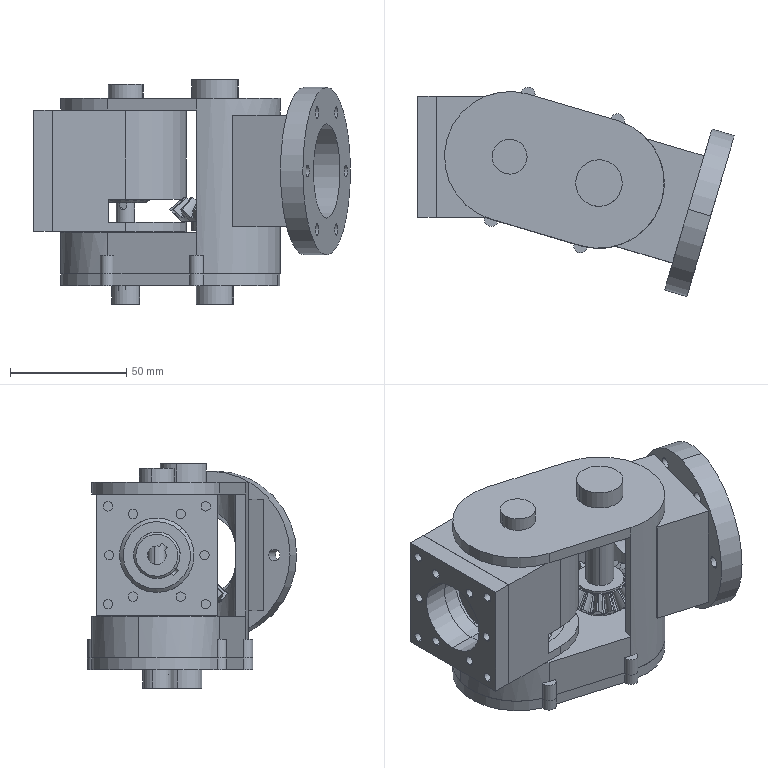Part | SolidWorks | features CompositeCurve 5 | 13 solids | 1270 faces | box 136.042 x 89.867 x 96.4 mm | volume 262623 mm3 | cylinder 494 | plane 308 | spline 304 | cone 160 | torus 4 | commonest cylinder face diameters 37.5 x82 42 x80 4 x44 0.475 x39 3 x30 0.375 x26